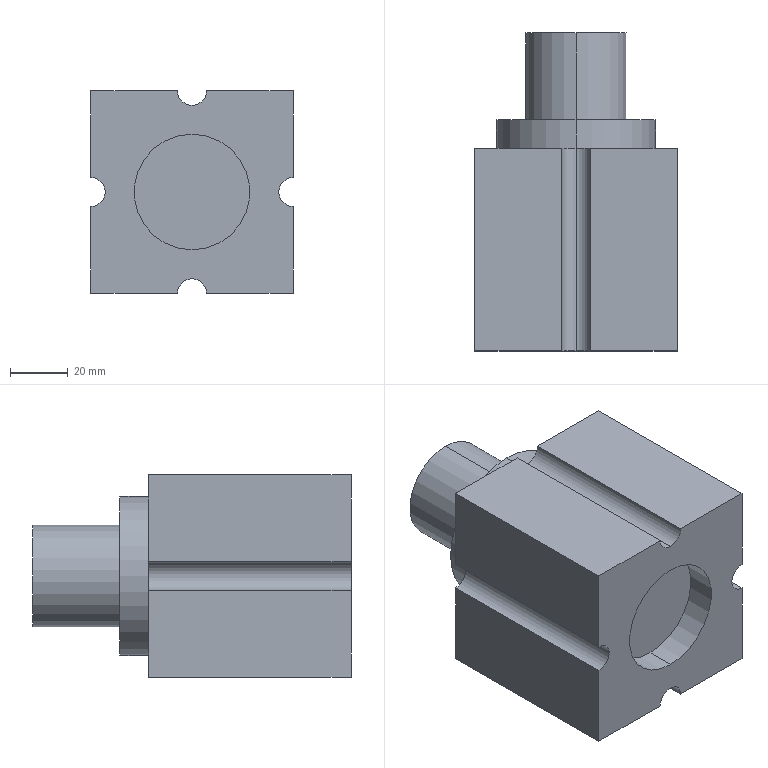Part | SolidWorks | features ICE 3, Extrusion 1 | 1 solid | 24 faces | box 70 x 110 x 70 mm | volume 372060 mm3 | plane 13 | cylinder 11 | commonest cylinder face diameters 10 x5 35 x2 40 x2 55 x2
STEP:
#1=CARTESIAN_POINT('',(0.,110.,17.5));
#2=VERTEX_POINT('',#1);
#3=CARTESIAN_POINT('',(0.,110.,-17.5));
#4=VERTEX_POINT('',#3);
#5=CARTESIAN_POINT('',(0.,110.,0.));
#6=DIRECTION('',(0.,1.,0.));
#7=DIRECTION('',(0.,0.,1.));
#8=AXIS2_PLACEMENT_3D('',#5,#6,#7);
#9=CIRCLE('',#8,17.5);
#10=EDGE_CURVE('',#2,#4,#9,.T.);
#11=ORIENTED_EDGE('',*,*,#10,.F.);
#12=CARTESIAN_POINT('',(0.,80.,17.5));
#13=VERTEX_POINT('',#12);
#14=CARTESIAN_POINT('',(0.,110.,17.5));
#15=DIRECTION('',(0.,-1.,0.));
#16=VECTOR('',#15,1000.);
#17=LINE('',#14,#16);
#18=EDGE_CURVE('',#2,#13,#17,.T.);
#19=ORIENTED_EDGE('',*,*,#18,.T.);
#20=CARTESIAN_POINT('',(0.,80.,-17.5));
#21=VERTEX_POINT('',#20);
#22=CARTESIAN_POINT('',(0.,80.,0.));
#23=DIRECTION('',(0.,1.,0.));
#24=DIRECTION('',(0.,0.,1.));
#25=AXIS2_PLACEMENT_3D('',#22,#23,#24);
#26=CIRCLE('',#25,17.5);
#27=EDGE_CURVE('',#13,#21,#26,.T.);
#28=ORIENTED_EDGE('',*,*,#27,.T.);
#29=CARTESIAN_POINT('',(0.,110.,-17.5));
#30=DIRECTION('',(0.,-1.,0.));
#31=VECTOR('',#30,1000.);
#32=LINE('',#29,#31);
#33=EDGE_CURVE('',#4,#21,#32,.T.);
#34=ORIENTED_EDGE('',*,*,#33,.F.);
#35=EDGE_LOOP('',(#11,#19,#28,#34));
#36=FACE_OUTER_BOUND('',#35,.T.);
#37=CARTESIAN_POINT('',(0.,110.,0.));
#38=DIRECTION('',(0.,-1.,0.));
#39=DIRECTION('',(0.,0.,-1.));
#40=AXIS2_PLACEMENT_3D('',#37,#38,#39);
#41=CYLINDRICAL_SURFACE('',#40,17.5);
#42=ADVANCED_FACE('',(#36),#41,.T.);
#43=CARTESIAN_POINT('',(0.,80.,27.5));
#44=VERTEX_POINT('',#43);
#45=CARTESIAN_POINT('',(0.,80.,-27.5));
#46=VERTEX_POINT('',#45);
#47=CARTESIAN_POINT('',(0.,80.,0.));
#48=DIRECTION('',(0.,1.,0.));
#49=DIRECTION('',(0.,0.,1.));
#50=AXIS2_PLACEMENT_3D('',#47,#48,#49);
#51=CIRCLE('',#50,27.5);
#52=EDGE_CURVE('',#44,#46,#51,.T.);
#53=ORIENTED_EDGE('',*,*,#52,.F.);
#54=CARTESIAN_POINT('',(0.,70.,27.5));
#55=VERTEX_POINT('',#54);
#56=CARTESIAN_POINT('',(0.,80.,27.5));
#57=DIRECTION('',(0.,-1.,0.));
#58=VECTOR('',#57,1000.);
#59=LINE('',#56,#58);
#60=EDGE_CURVE('',#44,#55,#59,.T.);
#61=ORIENTED_EDGE('',*,*,#60,.T.);
#62=CARTESIAN_POINT('',(0.,70.,-27.5));
#63=VERTEX_POINT('',#62);
#64=CARTESIAN_POINT('',(0.,70.,0.));
#65=DIRECTION('',(0.,1.,0.));
#66=DIRECTION('',(0.,0.,1.));
#67=AXIS2_PLACEMENT_3D('',#64,#65,#66);
#68=CIRCLE('',#67,27.5);
#69=EDGE_CURVE('',#55,#63,#68,.T.);
#70=ORIENTED_EDGE('',*,*,#69,.T.);
#71=CARTESIAN_POINT('',(0.,80.,-27.5));
#72=DIRECTION('',(0.,-1.,0.));
#73=VECTOR('',#72,1000.);
#74=LINE('',#71,#73);
#75=EDGE_CURVE('',#46,#63,#74,.T.);
#76=ORIENTED_EDGE('',*,*,#75,.F.);
#77=EDGE_LOOP('',(#53,#61,#70,#76));
#78=FACE_OUTER_BOUND('',#77,.T.);
#79=CARTESIAN_POINT('',(0.,80.,0.));
#80=DIRECTION('',(0.,-1.,0.));
#81=DIRECTION('',(0.,0.,-1.));
#82=AXIS2_PLACEMENT_3D('',#79,#80,#81);
#83=CYLINDRICAL_SURFACE('',#82,27.5);
#84=ADVANCED_FACE('',(#78),#83,.T.);
#85=CARTESIAN_POINT('',(0.,10.,20.));
#86=VERTEX_POINT('',#85);
#87=CARTESIAN_POINT('',(0.,10.,-20.));
#88=VERTEX_POINT('',#87);
#89=CARTESIAN_POINT('',(0.,10.,0.));
#90=DIRECTION('',(0.,-1.,0.));
#91=DIRECTION('',(0.,0.,-1.));
#92=AXIS2_PLACEMENT_3D('',#89,#90,#91);
#93=CIRCLE('',#92,20.);
#94=EDGE_CURVE('',#86,#88,#93,.T.);
#95=ORIENTED_EDGE('',*,*,#94,.F.);
#96=CARTESIAN_POINT('',(0.,0.,20.));
#97=VERTEX_POINT('',#96);
#98=CARTESIAN_POINT('',(0.,10.,20.));
#99=DIRECTION('',(0.,-1.,0.));
#100=VECTOR('',#99,1000.);
#101=LINE('',#98,#100);
#102=EDGE_CURVE('',#86,#97,#101,.T.);
#103=ORIENTED_EDGE('',*,*,#102,.T.);
#104=CARTESIAN_POINT('',(0.,0.,-20.));
#105=VERTEX_POINT('',#104);
#106=CARTESIAN_POINT('',(0.,0.,0.));
#107=DIRECTION('',(0.,-1.,0.));
#108=DIRECTION('',(0.,0.,-1.));
#109=AXIS2_PLACEMENT_3D('',#106,#107,#108);
#110=CIRCLE('',#109,20.);
#111=EDGE_CURVE('',#97,#105,#110,.T.);
#112=ORIENTED_EDGE('',*,*,#111,.T.);
#113=CARTESIAN_POINT('',(0.,10.,-20.));
#114=DIRECTION('',(0.,-1.,0.));
#115=VECTOR('',#114,1000.);
#116=LINE('',#113,#115);
#117=EDGE_CURVE('',#88,#105,#116,.T.);
#118=ORIENTED_EDGE('',*,*,#117,.F.);
#119=EDGE_LOOP('',(#95,#103,#112,#118));
#120=FACE_OUTER_BOUND('',#119,.T.);
#121=CARTESIAN_POINT('',(0.,10.,0.));
#122=DIRECTION('',(0.,-1.,0.));
#123=DIRECTION('',(0.,0.,-1.));
#124=AXIS2_PLACEMENT_3D('',#121,#122,#123);
#125=CYLINDRICAL_SURFACE('',#124,20.);
#126=ADVANCED_FACE('',(#120),#125,.F.);
#127=CARTESIAN_POINT('',(0.,70.,30.));
#128=VERTEX_POINT('',#127);
#129=CARTESIAN_POINT('',(5.,70.,35.));
#130=VERTEX_POINT('',#129);
#131=CARTESIAN_POINT('',(0.,70.,35.));
#132=DIRECTION('',(0.,-1.,0.));
#133=DIRECTION('',(0.,0.,1.));
#134=AXIS2_PLACEMENT_3D('',#131,#132,#133);
#135=CIRCLE('',#134,5.);
#136=EDGE_CURVE('',#128,#130,#135,.T.);
#137=ORIENTED_EDGE('',*,*,#136,.F.);
#138=CARTESIAN_POINT('',(0.,0.,30.));
#139=VERTEX_POINT('',#138);
#140=CARTESIAN_POINT('',(0.,70.,30.));
#141=DIRECTION('',(0.,-1.,0.));
#142=VECTOR('',#141,1000.);
#143=LINE('',#140,#142);
#144=EDGE_CURVE('',#128,#139,#143,.T.);
#145=ORIENTED_EDGE('',*,*,#144,.T.);
#146=CARTESIAN_POINT('',(5.,0.,35.));
#147=VERTEX_POINT('',#146);
#148=CARTESIAN_POINT('',(0.,0.,35.));
#149=DIRECTION('',(0.,-1.,0.));
#150=DIRECTION('',(0.,0.,1.));
#151=AXIS2_PLACEMENT_3D('',#148,#149,#150);
#152=CIRCLE('',#151,5.);
#153=EDGE_CURVE('',#139,#147,#152,.T.);
#154=ORIENTED_EDGE('',*,*,#153,.T.);
#155=CARTESIAN_POINT('',(5.,70.,35.));
#156=DIRECTION('',(0.,-1.,0.));
#157=VECTOR('',#156,1000.);
#158=LINE('',#155,#157);
#159=EDGE_CURVE('',#130,#147,#158,.T.);
#160=ORIENTED_EDGE('',*,*,#159,.F.);
#161=EDGE_LOOP('',(#137,#145,#154,#160));
#162=FACE_OUTER_BOUND('',#161,.T.);
#163=CARTESIAN_POINT('',(0.,70.,35.));
#164=DIRECTION('',(0.,-1.,0.));
#165=DIRECTION('',(0.,0.,-1.));
#166=AXIS2_PLACEMENT_3D('',#163,#164,#165);
#167=CYLINDRICAL_SURFACE('',#166,5.);
#168=ADVANCED_FACE('',(#162),#167,.F.);
#169=CARTESIAN_POINT('',(35.,0.,-5.));
#170=VERTEX_POINT('',#169);
#171=CARTESIAN_POINT('',(35.,0.,-35.));
#172=VERTEX_POINT('',#171);
#173=CARTESIAN_POINT('',(35.,0.,-5.));
#174=DIRECTION('',(0.,0.,-1.));
#175=VECTOR('',#174,1000.);
#176=LINE('',#173,#175);
#177=EDGE_CURVE('',#170,#172,#176,.T.);
#178=ORIENTED_EDGE('',*,*,#177,.T.);
#179=CARTESIAN_POINT('',(35.,70.,-35.));
#180=VERTEX_POINT('',#179);
#181=CARTESIAN_POINT('',(35.,70.,-35.));
#182=DIRECTION('',(0.,-1.,0.));
#183=VECTOR('',#182,1000.);
#184=LINE('',#181,#183);
#185=EDGE_CURVE('',#180,#172,#184,.T.);
#186=ORIENTED_EDGE('',*,*,#185,.F.);
#187=CARTESIAN_POINT('',(35.,70.,-5.));
#188=VERTEX_POINT('',#187);
#189=CARTESIAN_POINT('',(35.,70.,-5.));
#190=DIRECTION('',(0.,0.,-1.));
#191=VECTOR('',#190,1000.);
#192=LINE('',#189,#191);
#193=EDGE_CURVE('',#188,#180,#192,.T.);
#194=ORIENTED_EDGE('',*,*,#193,.F.);
#195=CARTESIAN_POINT('',(35.,70.,-5.));
#196=DIRECTION('',(0.,-1.,0.));
#197=VECTOR('',#196,1000.);
#198=LINE('',#195,#197);
#199=EDGE_CURVE('',#188,#170,#198,.T.);
#200=ORIENTED_EDGE('',*,*,#199,.T.);
#201=EDGE_LOOP('',(#178,#186,#194,#200));
#202=FACE_OUTER_BOUND('',#201,.T.);
#203=CARTESIAN_POINT('',(35.,70.,-5.));
#204=DIRECTION('',(-1.,0.,0.));
#205=DIRECTION('',(0.,0.,1.));
#206=AXIS2_PLACEMENT_3D('',#203,#204,#205);
#207=PLANE('',#206);
#208=ADVANCED_FACE('',(#202),#207,.F.);
#209=CARTESIAN_POINT('',(5.,0.,-35.));
#210=VERTEX_POINT('',#209);
#211=CARTESIAN_POINT('',(5.,0.,-35.));
#212=DIRECTION('',(-1.,0.,0.));
#213=VECTOR('',#212,1000.);
#214=LINE('',#211,#213);
#215=EDGE_CURVE('',#172,#210,#214,.T.);
#216=ORIENTED_EDGE('',*,*,#215,.T.);
#217=CARTESIAN_POINT('',(5.,70.,-35.));
#218=VERTEX_POINT('',#217);
#219=CARTESIAN_POINT('',(5.,70.,-35.));
#220=DIRECTION('',(0.,-1.,0.));
#221=VECTOR('',#220,1000.);
#222=LINE('',#219,#221);
#223=EDGE_CURVE('',#218,#210,#222,.T.);
#224=ORIENTED_EDGE('',*,*,#223,.F.);
#225=CARTESIAN_POINT('',(5.,70.,-35.));
#226=DIRECTION('',(-1.,0.,0.));
#227=VECTOR('',#226,1000.);
#228=LINE('',#225,#227);
#229=EDGE_CURVE('',#180,#218,#228,.T.);
#230=ORIENTED_EDGE('',*,*,#229,.F.);
#231=ORIENTED_EDGE('',*,*,#185,.T.);
#232=EDGE_LOOP('',(#216,#224,#230,#231));
#233=FACE_OUTER_BOUND('',#232,.T.);
#234=CARTESIAN_POINT('',(5.,70.,-35.));
#235=DIRECTION('',(0.,0.,1.));
#236=DIRECTION('',(1.,0.,0.));
#237=AXIS2_PLACEMENT_3D('',#234,#235,#236);
#238=PLANE('',#237);
#239=ADVANCED_FACE('',(#233),#238,.F.);
#240=CARTESIAN_POINT('',(-5.,0.,-35.));
#241=VERTEX_POINT('',#240);
#242=CARTESIAN_POINT('',(0.,0.,-35.));
#243=DIRECTION('',(0.,-1.,0.));
#244=DIRECTION('',(0.,0.,1.));
#245=AXIS2_PLACEMENT_3D('',#242,#243,#244);
#246=CIRCLE('',#245,5.);
#247=EDGE_CURVE('',#210,#241,#246,.T.);
#248=ORIENTED_EDGE('',*,*,#247,.T.);
#249=CARTESIAN_POINT('',(-5.,70.,-35.));
#250=VERTEX_POINT('',#249);
#251=CARTESIAN_POINT('',(-5.,70.,-35.));
#252=DIRECTION('',(0.,-1.,0.));
#253=VECTOR('',#252,1000.);
#254=LINE('',#251,#253);
#255=EDGE_CURVE('',#250,#241,#254,.T.);
#256=ORIENTED_EDGE('',*,*,#255,.F.);
#257=CARTESIAN_POINT('',(0.,70.,-35.));
#258=DIRECTION('',(0.,-1.,0.));
#259=DIRECTION('',(0.,0.,1.));
#260=AXIS2_PLACEMENT_3D('',#257,#258,#259);
#261=CIRCLE('',#260,5.);
#262=EDGE_CURVE('',#218,#250,#261,.T.);
#263=ORIENTED_EDGE('',*,*,#262,.F.);
#264=ORIENTED_EDGE('',*,*,#223,.T.);
#265=EDGE_LOOP('',(#248,#256,#263,#264));
#266=FACE_OUTER_BOUND('',#265,.T.);
#267=CARTESIAN_POINT('',(0.,70.,-35.));
#268=DIRECTION('',(0.,-1.,0.));
#269=DIRECTION('',(0.,0.,-1.));
#270=AXIS2_PLACEMENT_3D('',#267,#268,#269);
#271=CYLINDRICAL_SURFACE('',#270,5.);
#272=ADVANCED_FACE('',(#266),#271,.F.);
#273=CARTESIAN_POINT('',(-35.,0.,-35.));
#274=VERTEX_POINT('',#273);
#275=CARTESIAN_POINT('',(-35.,0.,-35.));
#276=DIRECTION('',(-1.,0.,0.));
#277=VECTOR('',#276,1000.);
#278=LINE('',#275,#277);
#279=EDGE_CURVE('',#241,#274,#278,.T.);
#280=ORIENTED_EDGE('',*,*,#279,.T.);
#281=CARTESIAN_POINT('',(-35.,70.,-35.));
#282=VERTEX_POINT('',#281);
#283=CARTESIAN_POINT('',(-35.,70.,-35.));
#284=DIRECTION('',(0.,-1.,0.));
#285=VECTOR('',#284,1000.);
#286=LINE('',#283,#285);
#287=EDGE_CURVE('',#282,#274,#286,.T.);
#288=ORIENTED_EDGE('',*,*,#287,.F.);
#289=CARTESIAN_POINT('',(-35.,70.,-35.));
#290=DIRECTION('',(-1.,0.,0.));
#291=VECTOR('',#290,1000.);
#292=LINE('',#289,#291);
#293=EDGE_CURVE('',#250,#282,#292,.T.);
#294=ORIENTED_EDGE('',*,*,#293,.F.);
#295=ORIENTED_EDGE('',*,*,#255,.T.);
#296=EDGE_LOOP('',(#280,#288,#294,#295));
#297=FACE_OUTER_BOUND('',#296,.T.);
#298=CARTESIAN_POINT('',(-35.,70.,-35.));
#299=DIRECTION('',(0.,0.,1.));
#300=DIRECTION('',(1.,0.,0.));
#301=AXIS2_PLACEMENT_3D('',#298,#299,#300);
#302=PLANE('',#301);
#303=ADVANCED_FACE('',(#297),#302,.F.);
#304=CARTESIAN_POINT('',(-35.,0.,-5.));
#305=VERTEX_POINT('',#304);
#306=CARTESIAN_POINT('',(-35.,0.,-5.));
#307=DIRECTION('',(0.,0.,1.));
#308=VECTOR('',#307,1000.);
#309=LINE('',#306,#308);
#310=EDGE_CURVE('',#274,#305,#309,.T.);
#311=ORIENTED_EDGE('',*,*,#310,.T.);
#312=CARTESIAN_POINT('',(-35.,70.,-5.));
#313=VERTEX_POINT('',#312);
#314=CARTESIAN_POINT('',(-35.,70.,-5.));
#315=DIRECTION('',(0.,-1.,0.));
#316=VECTOR('',#315,1000.);
#317=LINE('',#314,#316);
#318=EDGE_CURVE('',#313,#305,#317,.T.);
#319=ORIENTED_EDGE('',*,*,#318,.F.);
#320=CARTESIAN_POINT('',(-35.,70.,-5.));
#321=DIRECTION('',(0.,0.,1.));
#322=VECTOR('',#321,1000.);
#323=LINE('',#320,#322);
#324=EDGE_CURVE('',#282,#313,#323,.T.);
#325=ORIENTED_EDGE('',*,*,#324,.F.);
#326=ORIENTED_EDGE('',*,*,#287,.T.);
#327=EDGE_LOOP('',(#311,#319,#325,#326));
#328=FACE_OUTER_BOUND('',#327,.T.);
#329=CARTESIAN_POINT('',(-35.,70.,-5.));
#330=DIRECTION('',(1.,0.,0.));
#331=DIRECTION('',(0.,0.,-1.));
#332=AXIS2_PLACEMENT_3D('',#329,#330,#331);
#333=PLANE('',#332);
#334=ADVANCED_FACE('',(#328),#333,.F.);
#335=CARTESIAN_POINT('',(-35.,0.,5.));
#336=VERTEX_POINT('',#335);
#337=CARTESIAN_POINT('',(-35.,0.,0.));
#338=DIRECTION('',(0.,-1.,0.));
#339=DIRECTION('',(0.,0.,1.));
#340=AXIS2_PLACEMENT_3D('',#337,#338,#339);
#341=CIRCLE('',#340,5.);
#342=EDGE_CURVE('',#305,#336,#341,.T.);
#343=ORIENTED_EDGE('',*,*,#342,.T.);
#344=CARTESIAN_POINT('',(-35.,70.,5.));
#345=VERTEX_POINT('',#344);
#346=CARTESIAN_POINT('',(-35.,70.,5.));
#347=DIRECTION('',(0.,-1.,0.));
#348=VECTOR('',#347,1000.);
#349=LINE('',#346,#348);
#350=EDGE_CURVE('',#345,#336,#349,.T.);
#351=ORIENTED_EDGE('',*,*,#350,.F.);
#352=CARTESIAN_POINT('',(-35.,70.,0.));
#353=DIRECTION('',(0.,-1.,0.));
#354=DIRECTION('',(0.,0.,1.));
#355=AXIS2_PLACEMENT_3D('',#352,#353,#354);
#356=CIRCLE('',#355,5.);
#357=EDGE_CURVE('',#313,#345,#356,.T.);
#358=ORIENTED_EDGE('',*,*,#357,.F.);
#359=ORIENTED_EDGE('',*,*,#318,.T.);
#360=EDGE_LOOP('',(#343,#351,#358,#359));
#361=FACE_OUTER_BOUND('',#360,.T.);
#362=CARTESIAN_POINT('',(-35.,70.,0.));
#363=DIRECTION('',(0.,-1.,0.));
#364=DIRECTION('',(0.,0.,-1.));
#365=AXIS2_PLACEMENT_3D('',#362,#363,#364);
#366=CYLINDRICAL_SURFACE('',#365,5.);
#367=ADVANCED_FACE('',(#361),#366,.F.);
#368=CARTESIAN_POINT('',(-35.,0.,35.));
#369=VERTEX_POINT('',#368);
#370=CARTESIAN_POINT('',(-35.,0.,35.));
#371=DIRECTION('',(0.,0.,1.));
#372=VECTOR('',#371,1000.);
#373=LINE('',#370,#372);
#374=EDGE_CURVE('',#336,#369,#373,.T.);
#375=ORIENTED_EDGE('',*,*,#374,.T.);
#376=CARTESIAN_POINT('',(-35.,70.,35.));
#377=VERTEX_POINT('',#376);
#378=CARTESIAN_POINT('',(-35.,70.,35.));
#379=DIRECTION('',(0.,-1.,0.));
#380=VECTOR('',#379,1000.);
#381=LINE('',#378,#380);
#382=EDGE_CURVE('',#377,#369,#381,.T.);
#383=ORIENTED_EDGE('',*,*,#382,.F.);
#384=CARTESIAN_POINT('',(-35.,70.,35.));
#385=DIRECTION('',(0.,0.,1.));
#386=VECTOR('',#385,1000.);
#387=LINE('',#384,#386);
#388=EDGE_CURVE('',#345,#377,#387,.T.);
#389=ORIENTED_EDGE('',*,*,#388,.F.);
#390=ORIENTED_EDGE('',*,*,#350,.T.);
#391=EDGE_LOOP('',(#375,#383,#389,#390));
#392=FACE_OUTER_BOUND('',#391,.T.);
#393=CARTESIAN_POINT('',(-35.,70.,35.));
#394=DIRECTION('',(1.,0.,0.));
#395=DIRECTION('',(0.,0.,-1.));
#396=AXIS2_PLACEMENT_3D('',#393,#394,#395);
#397=PLANE('',#396);
#398=ADVANCED_FACE('',(#392),#397,.F.);
#399=CARTESIAN_POINT('',(-5.,0.,35.));
#400=VERTEX_POINT('',#399);
#401=CARTESIAN_POINT('',(-35.,0.,35.));
#402=DIRECTION('',(1.,0.,0.));
#403=VECTOR('',#402,1000.);
#404=LINE('',#401,#403);
#405=EDGE_CURVE('',#369,#400,#404,.T.);
#406=ORIENTED_EDGE('',*,*,#405,.T.);
#407=CARTESIAN_POINT('',(-5.,70.,35.));
#408=VERTEX_POINT('',#407);
#409=CARTESIAN_POINT('',(-5.,70.,35.));
#410=DIRECTION('',(0.,-1.,0.));
#411=VECTOR('',#410,1000.);
#412=LINE('',#409,#411);
#413=EDGE_CURVE('',#408,#400,#412,.T.);
#414=ORIENTED_EDGE('',*,*,#413,.F.);
#415=CARTESIAN_POINT('',(-35.,70.,35.));
#416=DIRECTION('',(1.,0.,0.));
#417=VECTOR('',#416,1000.);
#418=LINE('',#415,#417);
#419=EDGE_CURVE('',#377,#408,#418,.T.);
#420=ORIENTED_EDGE('',*,*,#419,.F.);
#421=ORIENTED_EDGE('',*,*,#382,.T.);
#422=EDGE_LOOP('',(#406,#414,#420,#421));
#423=FACE_OUTER_BOUND('',#422,.T.);
#424=CARTESIAN_POINT('',(-35.,70.,35.));
#425=DIRECTION('',(0.,0.,-1.));
#426=DIRECTION('',(-1.,0.,0.));
#427=AXIS2_PLACEMENT_3D('',#424,#425,#426);
#428=PLANE('',#427);
#429=ADVANCED_FACE('',(#423),#428,.F.);
#430=ORIENTED_EDGE('',*,*,#144,.F.);
#431=CARTESIAN_POINT('',(0.,70.,35.));
#432=DIRECTION('',(0.,-1.,0.));
#433=DIRECTION('',(0.,0.,1.));
#434=AXIS2_PLACEMENT_3D('',#431,#432,#433);
#435=CIRCLE('',#434,5.);
#436=EDGE_CURVE('',#408,#128,#435,.T.);
#437=ORIENTED_EDGE('',*,*,#436,.F.);
#438=ORIENTED_EDGE('',*,*,#413,.T.);
#439=CARTESIAN_POINT('',(0.,0.,35.));
#440=DIRECTION('',(0.,-1.,0.));
#441=DIRECTION('',(0.,0.,1.));
#442=AXIS2_PLACEMENT_3D('',#439,#440,#441);
#443=CIRCLE('',#442,5.);
#444=EDGE_CURVE('',#400,#139,#443,.T.);
#445=ORIENTED_EDGE('',*,*,#444,.T.);
#446=EDGE_LOOP('',(#430,#437,#438,#445));
#447=FACE_OUTER_BOUND('',#446,.T.);
#448=CARTESIAN_POINT('',(0.,70.,35.));
#449=DIRECTION('',(0.,-1.,0.));
#450=DIRECTION('',(0.,0.,-1.));
#451=AXIS2_PLACEMENT_3D('',#448,#449,#450);
#452=CYLINDRICAL_SURFACE('',#451,5.);
#453=ADVANCED_FACE('',(#447),#452,.F.);
#454=CARTESIAN_POINT('',(35.,0.,35.));
#455=VERTEX_POINT('',#454);
#456=CARTESIAN_POINT('',(5.,0.,35.));
#457=DIRECTION('',(1.,0.,0.));
#458=VECTOR('',#457,1000.);
#459=LINE('',#456,#458);
#460=EDGE_CURVE('',#147,#455,#459,.T.);
#461=ORIENTED_EDGE('',*,*,#460,.T.);
#462=CARTESIAN_POINT('',(35.,70.,35.));
#463=VERTEX_POINT('',#462);
#464=CARTESIAN_POINT('',(35.,70.,35.));
#465=DIRECTION('',(0.,-1.,0.));
#466=VECTOR('',#465,1000.);
#467=LINE('',#464,#466);
#468=EDGE_CURVE('',#463,#455,#467,.T.);
#469=ORIENTED_EDGE('',*,*,#468,.F.);
#470=CARTESIAN_POINT('',(5.,70.,35.));
#471=DIRECTION('',(1.,0.,0.));
#472=VECTOR('',#471,1000.);
#473=LINE('',#470,#472);
#474=EDGE_CURVE('',#130,#463,#473,.T.);
#475=ORIENTED_EDGE('',*,*,#474,.F.);
#476=ORIENTED_EDGE('',*,*,#159,.T.);
#477=EDGE_LOOP('',(#461,#469,#475,#476));
#478=FACE_OUTER_BOUND('',#477,.T.);
#479=CARTESIAN_POINT('',(5.,70.,35.));
#480=DIRECTION('',(0.,0.,-1.));
#481=DIRECTION('',(-1.,0.,0.));
#482=AXIS2_PLACEMENT_3D('',#479,#480,#481);
#483=PLANE('',#482);
#484=ADVANCED_FACE('',(#478),#483,.F.);
#485=CARTESIAN_POINT('',(35.,0.,5.));
#486=VERTEX_POINT('',#485);
#487=CARTESIAN_POINT('',(35.,0.,35.));
#488=DIRECTION('',(0.,0.,-1.));
#489=VECTOR('',#488,1000.);
#490=LINE('',#487,#489);
#491=EDGE_CURVE('',#455,#486,#490,.T.);
#492=ORIENTED_EDGE('',*,*,#491,.T.);
#493=CARTESIAN_POINT('',(35.,70.,5.));
#494=VERTEX_POINT('',#493);
#495=CARTESIAN_POINT('',(35.,70.,5.));
#496=DIRECTION('',(0.,-1.,0.));
#497=VECTOR('',#496,1000.);
#498=LINE('',#495,#497);
#499=EDGE_CURVE('',#494,#486,#498,.T.);
#500=ORIENTED_EDGE('',*,*,#499,.F.);
#501=CARTESIAN_POINT('',(35.,70.,35.));
#502=DIRECTION('',(0.,0.,-1.));
#503=VECTOR('',#502,1000.);
#504=LINE('',#501,#503);
#505=EDGE_CURVE('',#463,#494,#504,.T.);
#506=ORIENTED_EDGE('',*,*,#505,.F.);
#507=ORIENTED_EDGE('',*,*,#468,.T.);
#508=EDGE_LOOP('',(#492,#500,#506,#507));
#509=FACE_OUTER_BOUND('',#508,.T.);
#510=CARTESIAN_POINT('',(35.,70.,35.));
#511=DIRECTION('',(-1.,0.,0.));
#512=DIRECTION('',(0.,0.,1.));
#513=AXIS2_PLACEMENT_3D('',#510,#511,#512);
#514=PLANE('',#513);
#515=ADVANCED_FACE('',(#509),#514,.F.);
#516=CARTESIAN_POINT('',(35.,0.,0.));
#517=DIRECTION('',(0.,-1.,0.));
#518=DIRECTION('',(0.,0.,1.));
#519=AXIS2_PLACEMENT_3D('',#516,#517,#518);
#520=CIRCLE('',#519,5.);
#521=EDGE_CURVE('',#486,#170,#520,.T.);
#522=ORIENTED_EDGE('',*,*,#521,.T.);
#523=ORIENTED_EDGE('',*,*,#199,.F.);
#524=CARTESIAN_POINT('',(35.,70.,0.));
#525=DIRECTION('',(0.,-1.,0.));
#526=DIRECTION('',(0.,0.,1.));
#527=AXIS2_PLACEMENT_3D('',#524,#525,#526);
#528=CIRCLE('',#527,5.);
#529=EDGE_CURVE('',#494,#188,#528,.T.);
#530=ORIENTED_EDGE('',*,*,#529,.F.);
#531=ORIENTED_EDGE('',*,*,#499,.T.);
#532=EDGE_LOOP('',(#522,#523,#530,#531));
#533=FACE_OUTER_BOUND('',#532,.T.);
#534=CARTESIAN_POINT('',(35.,70.,0.));
#535=DIRECTION('',(0.,-1.,0.));
#536=DIRECTION('',(0.,0.,-1.));
#537=AXIS2_PLACEMENT_3D('',#534,#535,#536);
#538=CYLINDRICAL_SURFACE('',#537,5.);
#539=ADVANCED_FACE('',(#533),#538,.F.);
#540=CARTESIAN_POINT('',(0.,70.,0.));
#541=DIRECTION('',(0.,1.,0.));
#542=DIRECTION('',(0.,0.,1.));
#543=AXIS2_PLACEMENT_3D('',#540,#541,#542);
#544=CIRCLE('',#543,27.5);
#545=EDGE_CURVE('',#63,#55,#544,.T.);
#546=ORIENTED_EDGE('',*,*,#545,.F.);
#547=ORIENTED_EDGE('',*,*,#69,.F.);
#548=EDGE_LOOP('',(#546,#547));
#549=FACE_BOUND('',#548,.T.);
#550=ORIENTED_EDGE('',*,*,#193,.T.);
#551=ORIENTED_EDGE('',*,*,#229,.T.);
#552=ORIENTED_EDGE('',*,*,#262,.T.);
#553=ORIENTED_EDGE('',*,*,#293,.T.);
#554=ORIENTED_EDGE('',*,*,#324,.T.);
#555=ORIENTED_EDGE('',*,*,#357,.T.);
#556=ORIENTED_EDGE('',*,*,#388,.T.);
#557=ORIENTED_EDGE('',*,*,#419,.T.);
#558=ORIENTED_EDGE('',*,*,#436,.T.);
#559=ORIENTED_EDGE('',*,*,#136,.T.);
#560=ORIENTED_EDGE('',*,*,#474,.T.);
#561=ORIENTED_EDGE('',*,*,#505,.T.);
#562=ORIENTED_EDGE('',*,*,#529,.T.);
#563=EDGE_LOOP('',(#550,#551,#552,#553,#554,#555,#556,#557,#558,#559,#560,#561,#562));
#564=FACE_OUTER_BOUND('',#563,.T.);
#565=CARTESIAN_POINT('',(0.,70.,-35.));
#566=DIRECTION('',(0.,1.,0.));
#567=DIRECTION('',(0.,0.,1.));
#568=AXIS2_PLACEMENT_3D('',#565,#566,#567);
#569=PLANE('',#568);
#570=ADVANCED_FACE('',(#549,#564),#569,.T.);
#571=CARTESIAN_POINT('',(0.,0.,0.));
#572=DIRECTION('',(0.,-1.,0.));
#573=DIRECTION('',(0.,0.,-1.));
#574=AXIS2_PLACEMENT_3D('',#571,#572,#573);
#575=CIRCLE('',#574,20.);
#576=EDGE_CURVE('',#105,#97,#575,.T.);
#577=ORIENTED_EDGE('',*,*,#576,.F.);
#578=ORIENTED_EDGE('',*,*,#111,.F.);
#579=EDGE_LOOP('',(#577,#578));
#580=FACE_BOUND('',#579,.T.);
#581=ORIENTED_EDGE('',*,*,#177,.F.);
#582=ORIENTED_EDGE('',*,*,#521,.F.);
#583=ORIENTED_EDGE('',*,*,#491,.F.);
#584=ORIENTED_EDGE('',*,*,#460,.F.);
#585=ORIENTED_EDGE('',*,*,#153,.F.);
#586=ORIENTED_EDGE('',*,*,#444,.F.);
#587=ORIENTED_EDGE('',*,*,#405,.F.);
#588=ORIENTED_EDGE('',*,*,#374,.F.);
#589=ORIENTED_EDGE('',*,*,#342,.F.);
#590=ORIENTED_EDGE('',*,*,#310,.F.);
#591=ORIENTED_EDGE('',*,*,#279,.F.);
#592=ORIENTED_EDGE('',*,*,#247,.F.);
#593=ORIENTED_EDGE('',*,*,#215,.F.);
#594=EDGE_LOOP('',(#581,#582,#583,#584,#585,#586,#587,#588,#589,#590,#591,#592,#593));
#595=FACE_OUTER_BOUND('',#594,.T.);
#596=CARTESIAN_POINT('',(0.,0.,-35.));
#597=DIRECTION('',(0.,1.,0.));
#598=DIRECTION('',(0.,0.,1.));
#599=AXIS2_PLACEMENT_3D('',#596,#597,#598);
#600=PLANE('',#599);
#601=ADVANCED_FACE('',(#580,#595),#600,.F.);
#602=ORIENTED_EDGE('',*,*,#102,.F.);
#603=CARTESIAN_POINT('',(0.,10.,0.));
#604=DIRECTION('',(0.,-1.,0.));
#605=DIRECTION('',(0.,0.,-1.));
#606=AXIS2_PLACEMENT_3D('',#603,#604,#605);
#607=CIRCLE('',#606,20.);
#608=EDGE_CURVE('',#88,#86,#607,.T.);
#609=ORIENTED_EDGE('',*,*,#608,.F.);
#610=ORIENTED_EDGE('',*,*,#117,.T.);
#611=ORIENTED_EDGE('',*,*,#576,.T.);
#612=EDGE_LOOP('',(#602,#609,#610,#611));
#613=FACE_OUTER_BOUND('',#612,.T.);
#614=CARTESIAN_POINT('',(0.,10.,0.));
#615=DIRECTION('',(0.,-1.,0.));
#616=DIRECTION('',(0.,0.,-1.));
#617=AXIS2_PLACEMENT_3D('',#614,#615,#616);
#618=CYLINDRICAL_SURFACE('',#617,20.);
#619=ADVANCED_FACE('',(#613),#618,.F.);
#620=ORIENTED_EDGE('',*,*,#608,.T.);
#621=ORIENTED_EDGE('',*,*,#94,.T.);
#622=EDGE_LOOP('',(#620,#621));
#623=FACE_OUTER_BOUND('',#622,.T.);
#624=CARTESIAN_POINT('',(0.,10.,0.));
#625=DIRECTION('',(0.,-1.,0.));
#626=DIRECTION('',(0.,0.,-1.));
#627=AXIS2_PLACEMENT_3D('',#624,#625,#626);
#628=PLANE('',#627);
#629=ADVANCED_FACE('',(#623),#628,.T.);
#630=ORIENTED_EDGE('',*,*,#60,.F.);
#631=CARTESIAN_POINT('',(0.,80.,0.));
#632=DIRECTION('',(0.,1.,0.));
#633=DIRECTION('',(0.,0.,1.));
#634=AXIS2_PLACEMENT_3D('',#631,#632,#633);
#635=CIRCLE('',#634,27.5);
#636=EDGE_CURVE('',#46,#44,#635,.T.);
#637=ORIENTED_EDGE('',*,*,#636,.F.);
#638=ORIENTED_EDGE('',*,*,#75,.T.);
#639=ORIENTED_EDGE('',*,*,#545,.T.);
#640=EDGE_LOOP('',(#630,#637,#638,#639));
#641=FACE_OUTER_BOUND('',#640,.T.);
#642=CARTESIAN_POINT('',(0.,80.,0.));
#643=DIRECTION('',(0.,-1.,0.));
#644=DIRECTION('',(0.,0.,-1.));
#645=AXIS2_PLACEMENT_3D('',#642,#643,#644);
#646=CYLINDRICAL_SURFACE('',#645,27.5);
#647=ADVANCED_FACE('',(#641),#646,.T.);
#648=CARTESIAN_POINT('',(0.,80.,0.));
#649=DIRECTION('',(0.,1.,0.));
#650=DIRECTION('',(0.,0.,1.));
#651=AXIS2_PLACEMENT_3D('',#648,#649,#650);
#652=CIRCLE('',#651,17.5);
#653=EDGE_CURVE('',#21,#13,#652,.T.);
#654=ORIENTED_EDGE('',*,*,#653,.F.);
#655=ORIENTED_EDGE('',*,*,#27,.F.);
#656=EDGE_LOOP('',(#654,#655));
#657=FACE_BOUND('',#656,.T.);
#658=ORIENTED_EDGE('',*,*,#636,.T.);
#659=ORIENTED_EDGE('',*,*,#52,.T.);
#660=EDGE_LOOP('',(#658,#659));
#661=FACE_OUTER_BOUND('',#660,.T.);
#662=CARTESIAN_POINT('',(0.,80.,0.));
#663=DIRECTION('',(0.,1.,0.));
#664=DIRECTION('',(0.,0.,1.));
#665=AXIS2_PLACEMENT_3D('',#662,#663,#664);
#666=PLANE('',#665);
#667=ADVANCED_FACE('',(#657,#661),#666,.T.);
#668=ORIENTED_EDGE('',*,*,#18,.F.);
#669=CARTESIAN_POINT('',(0.,110.,0.));
#670=DIRECTION('',(0.,1.,0.));
#671=DIRECTION('',(0.,0.,1.));
#672=AXIS2_PLACEMENT_3D('',#669,#670,#671);
#673=CIRCLE('',#672,17.5);
#674=EDGE_CURVE('',#4,#2,#673,.T.);
#675=ORIENTED_EDGE('',*,*,#674,.F.);
#676=ORIENTED_EDGE('',*,*,#33,.T.);
#677=ORIENTED_EDGE('',*,*,#653,.T.);
#678=EDGE_LOOP('',(#668,#675,#676,#677));
#679=FACE_OUTER_BOUND('',#678,.T.);
#680=CARTESIAN_POINT('',(0.,110.,0.));
#681=DIRECTION('',(0.,-1.,0.));
#682=DIRECTION('',(0.,0.,-1.));
#683=AXIS2_PLACEMENT_3D('',#680,#681,#682);
#684=CYLINDRICAL_SURFACE('',#683,17.5);
#685=ADVANCED_FACE('',(#679),#684,.T.);
#686=ORIENTED_EDGE('',*,*,#674,.T.);
#687=ORIENTED_EDGE('',*,*,#10,.T.);
#688=EDGE_LOOP('',(#686,#687));
#689=FACE_OUTER_BOUND('',#688,.T.);
#690=CARTESIAN_POINT('',(0.,110.,0.));
#691=DIRECTION('',(0.,1.,0.));
#692=DIRECTION('',(0.,0.,1.));
#693=AXIS2_PLACEMENT_3D('',#690,#691,#692);
#694=PLANE('',#693);
#695=ADVANCED_FACE('',(#689),#694,.T.);
#696=CLOSED_SHELL('',(#42,#84,#126,#168,#208,#239,#272,#303,#334,#367,#398,#429,#453,#484,#515,#539,#570,#601,#619,#629,#647,#667,#685,#695));
#697=MANIFOLD_SOLID_BREP('',#696);
#698=CARTESIAN_POINT('',(0.,0.,0.));
#699=DIRECTION('',(0.,0.,1.));
#700=DIRECTION('',(1.,0.,0.));
#701=AXIS2_PLACEMENT_3D('',#698,#699,#700);
#702=(LENGTH_UNIT()NAMED_UNIT(*)SI_UNIT(.MILLI.,.METRE.));
#703=UNCERTAINTY_MEASURE_WITH_UNIT(LENGTH_MEASURE(0.00001),#702,'','');
#704=(NAMED_UNIT(*)PLANE_ANGLE_UNIT()SI_UNIT($,.RADIAN.));
#705=(NAMED_UNIT(*)SI_UNIT($,.STERADIAN.)SOLID_ANGLE_UNIT());
#706=(GEOMETRIC_REPRESENTATION_CONTEXT(3)GLOBAL_UNCERTAINTY_ASSIGNED_CONTEXT((#703))GLOBAL_UNIT_ASSIGNED_CONTEXT((#702,#704,#705))REPRESENTATION_CONTEXT('',''));
#707=ADVANCED_BREP_SHAPE_REPRESENTATION('',(#697,#701),#706);